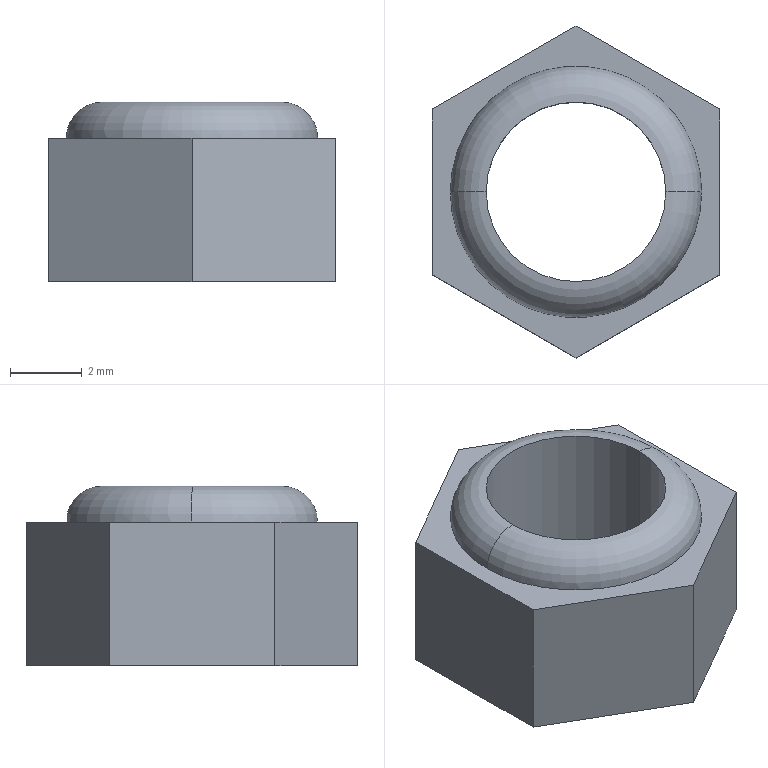Part | SolidWorks | features BaseBody 1 | 1 solid | 12 faces | box 8 x 9.238 x 5 mm | volume 157.594 mm3 | plane 8 | cylinder 2 | torus 2 | commonest cylinder face diameters 5 x2
STEP:
#1=CARTESIAN_POINT('',(2.5,0.,5.));
#2=VERTEX_POINT('',#1);
#3=CARTESIAN_POINT('',(-2.5,0.,5.));
#4=VERTEX_POINT('',#3);
#5=CARTESIAN_POINT('',(0.,0.,5.));
#6=DIRECTION('',(0.,0.,-1.));
#7=DIRECTION('',(-1.,0.,0.));
#8=AXIS2_PLACEMENT_3D('',#5,#6,#7);
#9=CIRCLE('',#8,2.5);
#10=EDGE_CURVE('',#2,#4,#9,.T.);
#11=ORIENTED_EDGE('',*,*,#10,.F.);
#12=CARTESIAN_POINT('',(2.5,0.,0.));
#13=VERTEX_POINT('',#12);
#14=CARTESIAN_POINT('',(2.5,0.,4.));
#15=DIRECTION('',(0.,0.,-1.));
#16=VECTOR('',#15,1000.);
#17=LINE('',#14,#16);
#18=EDGE_CURVE('',#2,#13,#17,.T.);
#19=ORIENTED_EDGE('',*,*,#18,.T.);
#20=CARTESIAN_POINT('',(-2.5,0.,0.));
#21=VERTEX_POINT('',#20);
#22=CARTESIAN_POINT('',(0.,0.,0.));
#23=DIRECTION('',(0.,0.,1.));
#24=DIRECTION('',(-1.,0.,0.));
#25=AXIS2_PLACEMENT_3D('',#22,#23,#24);
#26=CIRCLE('',#25,2.5);
#27=EDGE_CURVE('',#21,#13,#26,.T.);
#28=ORIENTED_EDGE('',*,*,#27,.F.);
#29=CARTESIAN_POINT('',(-2.5,0.,4.));
#30=DIRECTION('',(0.,0.,-1.));
#31=VECTOR('',#30,1000.);
#32=LINE('',#29,#31);
#33=EDGE_CURVE('',#4,#21,#32,.T.);
#34=ORIENTED_EDGE('',*,*,#33,.F.);
#35=EDGE_LOOP('',(#11,#19,#28,#34));
#36=FACE_OUTER_BOUND('',#35,.T.);
#37=CARTESIAN_POINT('',(0.,0.,4.));
#38=DIRECTION('',(0.,0.,-1.));
#39=DIRECTION('',(-1.,0.,0.));
#40=AXIS2_PLACEMENT_3D('',#37,#38,#39);
#41=CYLINDRICAL_SURFACE('',#40,2.5);
#42=ADVANCED_FACE('',(#36),#41,.F.);
#43=CARTESIAN_POINT('',(3.5,0.,4.));
#44=VERTEX_POINT('',#43);
#45=CARTESIAN_POINT('',(-3.5,0.,4.));
#46=VERTEX_POINT('',#45);
#47=CARTESIAN_POINT('',(0.,0.,4.));
#48=DIRECTION('',(0.,0.,1.));
#49=DIRECTION('',(1.,0.,0.));
#50=AXIS2_PLACEMENT_3D('',#47,#48,#49);
#51=CIRCLE('',#50,3.5);
#52=EDGE_CURVE('',#44,#46,#51,.T.);
#53=ORIENTED_EDGE('',*,*,#52,.T.);
#54=CARTESIAN_POINT('',(-2.5,0.,4.));
#55=DIRECTION('',(0.,1.,0.));
#56=DIRECTION('',(-1.,0.,0.));
#57=AXIS2_PLACEMENT_3D('',#54,#55,#56);
#58=CIRCLE('',#57,1.);
#59=EDGE_CURVE('',#46,#4,#58,.T.);
#60=ORIENTED_EDGE('',*,*,#59,.T.);
#61=CARTESIAN_POINT('',(0.,0.,5.));
#62=DIRECTION('',(0.,0.,-1.));
#63=DIRECTION('',(-1.,0.,0.));
#64=AXIS2_PLACEMENT_3D('',#61,#62,#63);
#65=CIRCLE('',#64,2.5);
#66=EDGE_CURVE('',#4,#2,#65,.T.);
#67=ORIENTED_EDGE('',*,*,#66,.T.);
#68=CARTESIAN_POINT('',(2.5,0.,4.));
#69=DIRECTION('',(0.,-1.,0.));
#70=DIRECTION('',(0.,0.,-1.));
#71=AXIS2_PLACEMENT_3D('',#68,#69,#70);
#72=CIRCLE('',#71,1.);
#73=EDGE_CURVE('',#44,#2,#72,.T.);
#74=ORIENTED_EDGE('',*,*,#73,.F.);
#75=EDGE_LOOP('',(#53,#60,#67,#74));
#76=FACE_OUTER_BOUND('',#75,.T.);
#77=CARTESIAN_POINT('',(0.,0.,4.));
#78=DIRECTION('',(0.,0.,1.));
#79=DIRECTION('',(1.,0.,0.));
#80=AXIS2_PLACEMENT_3D('',#77,#78,#79);
#81=TOROIDAL_SURFACE('',#80,2.5,1.);
#82=ADVANCED_FACE('',(#76),#81,.T.);
#83=ORIENTED_EDGE('',*,*,#18,.F.);
#84=ORIENTED_EDGE('',*,*,#66,.F.);
#85=ORIENTED_EDGE('',*,*,#33,.T.);
#86=CARTESIAN_POINT('',(0.,0.,0.));
#87=DIRECTION('',(0.,0.,1.));
#88=DIRECTION('',(-1.,0.,0.));
#89=AXIS2_PLACEMENT_3D('',#86,#87,#88);
#90=CIRCLE('',#89,2.5);
#91=EDGE_CURVE('',#13,#21,#90,.T.);
#92=ORIENTED_EDGE('',*,*,#91,.F.);
#93=EDGE_LOOP('',(#83,#84,#85,#92));
#94=FACE_OUTER_BOUND('',#93,.T.);
#95=CARTESIAN_POINT('',(0.,0.,4.));
#96=DIRECTION('',(0.,0.,-1.));
#97=DIRECTION('',(-1.,0.,0.));
#98=AXIS2_PLACEMENT_3D('',#95,#96,#97);
#99=CYLINDRICAL_SURFACE('',#98,2.5);
#100=ADVANCED_FACE('',(#94),#99,.F.);
#101=ORIENTED_EDGE('',*,*,#59,.F.);
#102=CARTESIAN_POINT('',(0.,0.,4.));
#103=DIRECTION('',(0.,0.,1.));
#104=DIRECTION('',(1.,0.,0.));
#105=AXIS2_PLACEMENT_3D('',#102,#103,#104);
#106=CIRCLE('',#105,3.5);
#107=EDGE_CURVE('',#46,#44,#106,.T.);
#108=ORIENTED_EDGE('',*,*,#107,.T.);
#109=ORIENTED_EDGE('',*,*,#73,.T.);
#110=ORIENTED_EDGE('',*,*,#10,.T.);
#111=EDGE_LOOP('',(#101,#108,#109,#110));
#112=FACE_OUTER_BOUND('',#111,.T.);
#113=CARTESIAN_POINT('',(0.,0.,4.));
#114=DIRECTION('',(0.,0.,1.));
#115=DIRECTION('',(1.,0.,0.));
#116=AXIS2_PLACEMENT_3D('',#113,#114,#115);
#117=TOROIDAL_SURFACE('',#116,2.5,1.);
#118=ADVANCED_FACE('',(#112),#117,.T.);
#119=CARTESIAN_POINT('',(0.,-4.619,0.));
#120=VERTEX_POINT('',#119);
#121=CARTESIAN_POINT('',(4.,-2.309,0.));
#122=VERTEX_POINT('',#121);
#123=CARTESIAN_POINT('',(0.,-4.619,0.));
#124=DIRECTION('',(0.866,0.5,0.));
#125=VECTOR('',#124,1000.);
#126=LINE('',#123,#125);
#127=EDGE_CURVE('',#120,#122,#126,.T.);
#128=ORIENTED_EDGE('',*,*,#127,.F.);
#129=CARTESIAN_POINT('',(-4.,-2.309,0.));
#130=VERTEX_POINT('',#129);
#131=CARTESIAN_POINT('',(-4.,-2.309,0.));
#132=DIRECTION('',(0.866,-0.5,0.));
#133=VECTOR('',#132,1000.);
#134=LINE('',#131,#133);
#135=EDGE_CURVE('',#130,#120,#134,.T.);
#136=ORIENTED_EDGE('',*,*,#135,.F.);
#137=CARTESIAN_POINT('',(-4.,2.309,0.));
#138=VERTEX_POINT('',#137);
#139=CARTESIAN_POINT('',(-4.,0.,0.));
#140=DIRECTION('',(0.,-1.,0.));
#141=VECTOR('',#140,1000.);
#142=LINE('',#139,#141);
#143=EDGE_CURVE('',#138,#130,#142,.T.);
#144=ORIENTED_EDGE('',*,*,#143,.F.);
#145=CARTESIAN_POINT('',(0.,4.619,0.));
#146=VERTEX_POINT('',#145);
#147=CARTESIAN_POINT('',(0.,4.619,0.));
#148=DIRECTION('',(-0.866,-0.5,0.));
#149=VECTOR('',#148,1000.);
#150=LINE('',#147,#149);
#151=EDGE_CURVE('',#146,#138,#150,.T.);
#152=ORIENTED_EDGE('',*,*,#151,.F.);
#153=CARTESIAN_POINT('',(4.,2.309,0.));
#154=VERTEX_POINT('',#153);
#155=CARTESIAN_POINT('',(4.,2.309,0.));
#156=DIRECTION('',(-0.866,0.5,0.));
#157=VECTOR('',#156,1000.);
#158=LINE('',#155,#157);
#159=EDGE_CURVE('',#154,#146,#158,.T.);
#160=ORIENTED_EDGE('',*,*,#159,.F.);
#161=CARTESIAN_POINT('',(4.,0.,0.));
#162=DIRECTION('',(0.,1.,0.));
#163=VECTOR('',#162,1000.);
#164=LINE('',#161,#163);
#165=EDGE_CURVE('',#122,#154,#164,.T.);
#166=ORIENTED_EDGE('',*,*,#165,.F.);
#167=EDGE_LOOP('',(#128,#136,#144,#152,#160,#166));
#168=FACE_OUTER_BOUND('',#167,.T.);
#169=ORIENTED_EDGE('',*,*,#27,.T.);
#170=ORIENTED_EDGE('',*,*,#91,.T.);
#171=EDGE_LOOP('',(#169,#170));
#172=FACE_BOUND('',#171,.T.);
#173=CARTESIAN_POINT('',(0.,0.,0.));
#174=DIRECTION('',(0.,0.,1.));
#175=DIRECTION('',(1.,0.,0.));
#176=AXIS2_PLACEMENT_3D('',#173,#174,#175);
#177=PLANE('',#176);
#178=ADVANCED_FACE('',(#168,#172),#177,.F.);
#179=CARTESIAN_POINT('',(-4.,2.309,4.));
#180=VERTEX_POINT('',#179);
#181=CARTESIAN_POINT('',(-4.,-2.309,4.));
#182=VERTEX_POINT('',#181);
#183=CARTESIAN_POINT('',(-4.,0.,4.));
#184=DIRECTION('',(0.,-1.,0.));
#185=VECTOR('',#184,1000.);
#186=LINE('',#183,#185);
#187=EDGE_CURVE('',#180,#182,#186,.T.);
#188=ORIENTED_EDGE('',*,*,#187,.T.);
#189=CARTESIAN_POINT('',(0.,-4.619,4.));
#190=VERTEX_POINT('',#189);
#191=CARTESIAN_POINT('',(-4.,-2.309,4.));
#192=DIRECTION('',(0.866,-0.5,0.));
#193=VECTOR('',#192,1000.);
#194=LINE('',#191,#193);
#195=EDGE_CURVE('',#182,#190,#194,.T.);
#196=ORIENTED_EDGE('',*,*,#195,.T.);
#197=CARTESIAN_POINT('',(4.,-2.309,4.));
#198=VERTEX_POINT('',#197);
#199=CARTESIAN_POINT('',(0.,-4.619,4.));
#200=DIRECTION('',(0.866,0.5,0.));
#201=VECTOR('',#200,1000.);
#202=LINE('',#199,#201);
#203=EDGE_CURVE('',#190,#198,#202,.T.);
#204=ORIENTED_EDGE('',*,*,#203,.T.);
#205=CARTESIAN_POINT('',(4.,2.309,4.));
#206=VERTEX_POINT('',#205);
#207=CARTESIAN_POINT('',(4.,0.,4.));
#208=DIRECTION('',(0.,1.,0.));
#209=VECTOR('',#208,1000.);
#210=LINE('',#207,#209);
#211=EDGE_CURVE('',#198,#206,#210,.T.);
#212=ORIENTED_EDGE('',*,*,#211,.T.);
#213=CARTESIAN_POINT('',(0.,4.619,4.));
#214=VERTEX_POINT('',#213);
#215=CARTESIAN_POINT('',(4.,2.309,4.));
#216=DIRECTION('',(-0.866,0.5,0.));
#217=VECTOR('',#216,1000.);
#218=LINE('',#215,#217);
#219=EDGE_CURVE('',#206,#214,#218,.T.);
#220=ORIENTED_EDGE('',*,*,#219,.T.);
#221=CARTESIAN_POINT('',(0.,4.619,4.));
#222=DIRECTION('',(-0.866,-0.5,0.));
#223=VECTOR('',#222,1000.);
#224=LINE('',#221,#223);
#225=EDGE_CURVE('',#214,#180,#224,.T.);
#226=ORIENTED_EDGE('',*,*,#225,.T.);
#227=EDGE_LOOP('',(#188,#196,#204,#212,#220,#226));
#228=FACE_OUTER_BOUND('',#227,.T.);
#229=ORIENTED_EDGE('',*,*,#52,.F.);
#230=ORIENTED_EDGE('',*,*,#107,.F.);
#231=EDGE_LOOP('',(#229,#230));
#232=FACE_BOUND('',#231,.T.);
#233=CARTESIAN_POINT('',(0.,0.,4.));
#234=DIRECTION('',(0.,0.,1.));
#235=DIRECTION('',(1.,0.,0.));
#236=AXIS2_PLACEMENT_3D('',#233,#234,#235);
#237=PLANE('',#236);
#238=ADVANCED_FACE('',(#228,#232),#237,.T.);
#239=ORIENTED_EDGE('',*,*,#211,.F.);
#240=CARTESIAN_POINT('',(4.,-2.309,4.));
#241=DIRECTION('',(0.,0.,1.));
#242=VECTOR('',#241,1000.);
#243=LINE('',#240,#242);
#244=EDGE_CURVE('',#122,#198,#243,.T.);
#245=ORIENTED_EDGE('',*,*,#244,.F.);
#246=ORIENTED_EDGE('',*,*,#165,.T.);
#247=CARTESIAN_POINT('',(4.,2.309,4.));
#248=DIRECTION('',(0.,0.,-1.));
#249=VECTOR('',#248,1000.);
#250=LINE('',#247,#249);
#251=EDGE_CURVE('',#206,#154,#250,.T.);
#252=ORIENTED_EDGE('',*,*,#251,.F.);
#253=EDGE_LOOP('',(#239,#245,#246,#252));
#254=FACE_OUTER_BOUND('',#253,.T.);
#255=CARTESIAN_POINT('',(4.,-2.309,4.));
#256=DIRECTION('',(-1.,0.,0.));
#257=DIRECTION('',(0.,0.,1.));
#258=AXIS2_PLACEMENT_3D('',#255,#256,#257);
#259=PLANE('',#258);
#260=ADVANCED_FACE('',(#254),#259,.F.);
#261=ORIENTED_EDGE('',*,*,#203,.F.);
#262=CARTESIAN_POINT('',(0.,-4.619,4.));
#263=DIRECTION('',(0.,0.,1.));
#264=VECTOR('',#263,1000.);
#265=LINE('',#262,#264);
#266=EDGE_CURVE('',#120,#190,#265,.T.);
#267=ORIENTED_EDGE('',*,*,#266,.F.);
#268=ORIENTED_EDGE('',*,*,#127,.T.);
#269=ORIENTED_EDGE('',*,*,#244,.T.);
#270=EDGE_LOOP('',(#261,#267,#268,#269));
#271=FACE_OUTER_BOUND('',#270,.T.);
#272=CARTESIAN_POINT('',(0.,-4.619,4.));
#273=DIRECTION('',(-0.5,0.866,0.));
#274=DIRECTION('',(-0.866,-0.5,0.));
#275=AXIS2_PLACEMENT_3D('',#272,#273,#274);
#276=PLANE('',#275);
#277=ADVANCED_FACE('',(#271),#276,.F.);
#278=ORIENTED_EDGE('',*,*,#195,.F.);
#279=CARTESIAN_POINT('',(-4.,-2.309,4.));
#280=DIRECTION('',(0.,0.,1.));
#281=VECTOR('',#280,1000.);
#282=LINE('',#279,#281);
#283=EDGE_CURVE('',#130,#182,#282,.T.);
#284=ORIENTED_EDGE('',*,*,#283,.F.);
#285=ORIENTED_EDGE('',*,*,#135,.T.);
#286=ORIENTED_EDGE('',*,*,#266,.T.);
#287=EDGE_LOOP('',(#278,#284,#285,#286));
#288=FACE_OUTER_BOUND('',#287,.T.);
#289=CARTESIAN_POINT('',(-4.,-2.309,4.));
#290=DIRECTION('',(0.5,0.866,0.));
#291=DIRECTION('',(-0.866,0.5,0.));
#292=AXIS2_PLACEMENT_3D('',#289,#290,#291);
#293=PLANE('',#292);
#294=ADVANCED_FACE('',(#288),#293,.F.);
#295=ORIENTED_EDGE('',*,*,#187,.F.);
#296=CARTESIAN_POINT('',(-4.,2.309,4.));
#297=DIRECTION('',(0.,0.,1.));
#298=VECTOR('',#297,1000.);
#299=LINE('',#296,#298);
#300=EDGE_CURVE('',#138,#180,#299,.T.);
#301=ORIENTED_EDGE('',*,*,#300,.F.);
#302=ORIENTED_EDGE('',*,*,#143,.T.);
#303=ORIENTED_EDGE('',*,*,#283,.T.);
#304=EDGE_LOOP('',(#295,#301,#302,#303));
#305=FACE_OUTER_BOUND('',#304,.T.);
#306=CARTESIAN_POINT('',(-4.,2.309,4.));
#307=DIRECTION('',(1.,0.,0.));
#308=DIRECTION('',(0.,0.,-1.));
#309=AXIS2_PLACEMENT_3D('',#306,#307,#308);
#310=PLANE('',#309);
#311=ADVANCED_FACE('',(#305),#310,.F.);
#312=ORIENTED_EDGE('',*,*,#225,.F.);
#313=CARTESIAN_POINT('',(0.,4.619,4.));
#314=DIRECTION('',(0.,0.,1.));
#315=VECTOR('',#314,1000.);
#316=LINE('',#313,#315);
#317=EDGE_CURVE('',#146,#214,#316,.T.);
#318=ORIENTED_EDGE('',*,*,#317,.F.);
#319=ORIENTED_EDGE('',*,*,#151,.T.);
#320=ORIENTED_EDGE('',*,*,#300,.T.);
#321=EDGE_LOOP('',(#312,#318,#319,#320));
#322=FACE_OUTER_BOUND('',#321,.T.);
#323=CARTESIAN_POINT('',(0.,4.619,4.));
#324=DIRECTION('',(0.5,-0.866,0.));
#325=DIRECTION('',(0.866,0.5,0.));
#326=AXIS2_PLACEMENT_3D('',#323,#324,#325);
#327=PLANE('',#326);
#328=ADVANCED_FACE('',(#322),#327,.F.);
#329=ORIENTED_EDGE('',*,*,#219,.F.);
#330=ORIENTED_EDGE('',*,*,#251,.T.);
#331=ORIENTED_EDGE('',*,*,#159,.T.);
#332=ORIENTED_EDGE('',*,*,#317,.T.);
#333=EDGE_LOOP('',(#329,#330,#331,#332));
#334=FACE_OUTER_BOUND('',#333,.T.);
#335=CARTESIAN_POINT('',(4.,2.309,4.));
#336=DIRECTION('',(-0.5,-0.866,0.));
#337=DIRECTION('',(0.866,-0.5,0.));
#338=AXIS2_PLACEMENT_3D('',#335,#336,#337);
#339=PLANE('',#338);
#340=ADVANCED_FACE('',(#334),#339,.F.);
#341=CLOSED_SHELL('',(#42,#82,#100,#118,#178,#238,#260,#277,#294,#311,#328,#340));
#342=MANIFOLD_SOLID_BREP('',#341);
#343=CARTESIAN_POINT('',(0.,0.,0.));
#344=DIRECTION('',(0.,0.,1.));
#345=DIRECTION('',(1.,0.,0.));
#346=AXIS2_PLACEMENT_3D('',#343,#344,#345);
#347=(LENGTH_UNIT()NAMED_UNIT(*)SI_UNIT(.MILLI.,.METRE.));
#348=UNCERTAINTY_MEASURE_WITH_UNIT(LENGTH_MEASURE(0.00001),#347,'','');
#349=(NAMED_UNIT(*)PLANE_ANGLE_UNIT()SI_UNIT($,.RADIAN.));
#350=(NAMED_UNIT(*)SI_UNIT($,.STERADIAN.)SOLID_ANGLE_UNIT());
#351=(GEOMETRIC_REPRESENTATION_CONTEXT(3)GLOBAL_UNCERTAINTY_ASSIGNED_CONTEXT((#348))GLOBAL_UNIT_ASSIGNED_CONTEXT((#347,#349,#350))REPRESENTATION_CONTEXT('',''));
#352=ADVANCED_BREP_SHAPE_REPRESENTATION('',(#342,#346),#351);